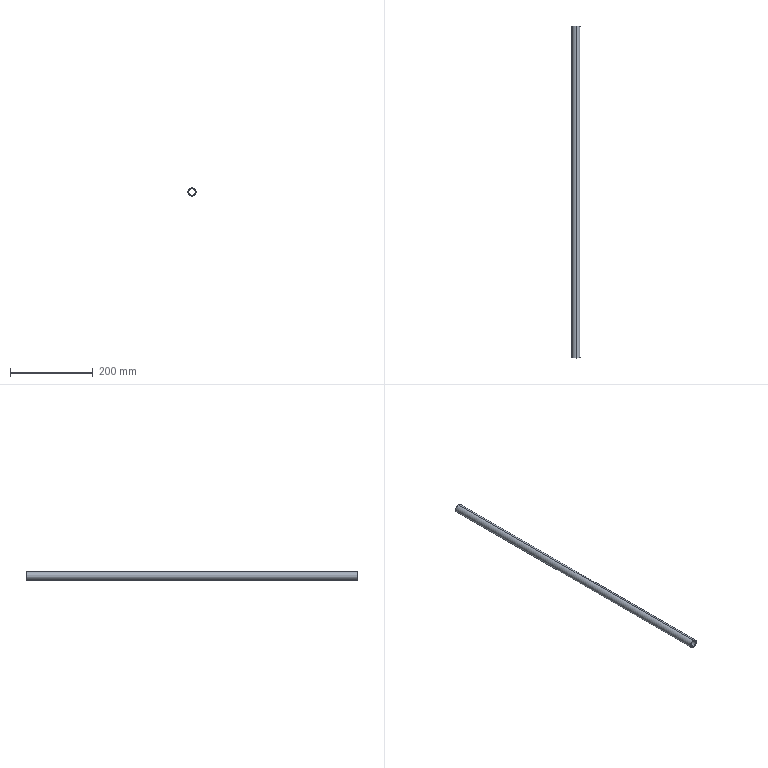Part | SolidWorks | features Sweep 1 | 1 solid | 6 faces | box 20 x 800 x 20 mm | volume 90478 mm3 | cylinder 4 | plane 2 | commonest cylinder face diameters 16 x2 20 x2
STEP:
#1=CARTESIAN_POINT('',(0.,0.,-8.));
#2=VERTEX_POINT('',#1);
#3=CARTESIAN_POINT('',(0.,0.,8.));
#4=VERTEX_POINT('',#3);
#5=CARTESIAN_POINT('',(0.,0.,0.));
#6=DIRECTION('',(0.,1.,0.));
#7=DIRECTION('',(0.,0.,1.));
#8=AXIS2_PLACEMENT_3D('',#5,#6,#7);
#9=CIRCLE('',#8,8.);
#10=EDGE_CURVE('',#2,#4,#9,.T.);
#11=ORIENTED_EDGE('',*,*,#10,.F.);
#12=CARTESIAN_POINT('',(0.,800.,-8.));
#13=VERTEX_POINT('',#12);
#14=CARTESIAN_POINT('',(0.,0.,-8.));
#15=DIRECTION('',(0.,1.,0.));
#16=VECTOR('',#15,1000.);
#17=LINE('',#14,#16);
#18=EDGE_CURVE('',#2,#13,#17,.T.);
#19=ORIENTED_EDGE('',*,*,#18,.T.);
#20=CARTESIAN_POINT('',(0.,800.,8.));
#21=VERTEX_POINT('',#20);
#22=CARTESIAN_POINT('',(0.,800.,0.));
#23=DIRECTION('',(0.,1.,0.));
#24=DIRECTION('',(0.,0.,1.));
#25=AXIS2_PLACEMENT_3D('',#22,#23,#24);
#26=CIRCLE('',#25,8.);
#27=EDGE_CURVE('',#13,#21,#26,.T.);
#28=ORIENTED_EDGE('',*,*,#27,.T.);
#29=CARTESIAN_POINT('',(0.,0.,8.));
#30=DIRECTION('',(0.,1.,0.));
#31=VECTOR('',#30,1000.);
#32=LINE('',#29,#31);
#33=EDGE_CURVE('',#4,#21,#32,.T.);
#34=ORIENTED_EDGE('',*,*,#33,.F.);
#35=EDGE_LOOP('',(#11,#19,#28,#34));
#36=FACE_OUTER_BOUND('',#35,.T.);
#37=CARTESIAN_POINT('',(0.,0.,0.));
#38=DIRECTION('',(0.,1.,0.));
#39=DIRECTION('',(0.,0.,1.));
#40=AXIS2_PLACEMENT_3D('',#37,#38,#39);
#41=CYLINDRICAL_SURFACE('',#40,8.);
#42=ADVANCED_FACE('',(#36),#41,.F.);
#43=CARTESIAN_POINT('',(0.,0.,10.));
#44=VERTEX_POINT('',#43);
#45=CARTESIAN_POINT('',(0.,0.,-10.));
#46=VERTEX_POINT('',#45);
#47=CARTESIAN_POINT('',(0.,0.,0.));
#48=DIRECTION('',(0.,1.,0.));
#49=DIRECTION('',(0.,0.,1.));
#50=AXIS2_PLACEMENT_3D('',#47,#48,#49);
#51=CIRCLE('',#50,10.);
#52=EDGE_CURVE('',#44,#46,#51,.T.);
#53=ORIENTED_EDGE('',*,*,#52,.T.);
#54=CARTESIAN_POINT('',(0.,800.,-10.));
#55=VERTEX_POINT('',#54);
#56=CARTESIAN_POINT('',(0.,0.,-10.));
#57=DIRECTION('',(0.,1.,0.));
#58=VECTOR('',#57,1000.);
#59=LINE('',#56,#58);
#60=EDGE_CURVE('',#46,#55,#59,.T.);
#61=ORIENTED_EDGE('',*,*,#60,.T.);
#62=CARTESIAN_POINT('',(0.,800.,10.));
#63=VERTEX_POINT('',#62);
#64=CARTESIAN_POINT('',(0.,800.,0.));
#65=DIRECTION('',(0.,1.,0.));
#66=DIRECTION('',(0.,0.,1.));
#67=AXIS2_PLACEMENT_3D('',#64,#65,#66);
#68=CIRCLE('',#67,10.);
#69=EDGE_CURVE('',#63,#55,#68,.T.);
#70=ORIENTED_EDGE('',*,*,#69,.F.);
#71=CARTESIAN_POINT('',(0.,0.,10.));
#72=DIRECTION('',(0.,1.,0.));
#73=VECTOR('',#72,1000.);
#74=LINE('',#71,#73);
#75=EDGE_CURVE('',#44,#63,#74,.T.);
#76=ORIENTED_EDGE('',*,*,#75,.F.);
#77=EDGE_LOOP('',(#53,#61,#70,#76));
#78=FACE_OUTER_BOUND('',#77,.T.);
#79=CARTESIAN_POINT('',(0.,0.,0.));
#80=DIRECTION('',(0.,1.,0.));
#81=DIRECTION('',(0.,0.,1.));
#82=AXIS2_PLACEMENT_3D('',#79,#80,#81);
#83=CYLINDRICAL_SURFACE('',#82,10.);
#84=ADVANCED_FACE('',(#78),#83,.T.);
#85=ORIENTED_EDGE('',*,*,#60,.F.);
#86=CARTESIAN_POINT('',(0.,0.,0.));
#87=DIRECTION('',(0.,1.,0.));
#88=DIRECTION('',(0.,0.,1.));
#89=AXIS2_PLACEMENT_3D('',#86,#87,#88);
#90=CIRCLE('',#89,10.);
#91=EDGE_CURVE('',#46,#44,#90,.T.);
#92=ORIENTED_EDGE('',*,*,#91,.T.);
#93=ORIENTED_EDGE('',*,*,#75,.T.);
#94=CARTESIAN_POINT('',(0.,800.,0.));
#95=DIRECTION('',(0.,1.,0.));
#96=DIRECTION('',(0.,0.,1.));
#97=AXIS2_PLACEMENT_3D('',#94,#95,#96);
#98=CIRCLE('',#97,10.);
#99=EDGE_CURVE('',#55,#63,#98,.T.);
#100=ORIENTED_EDGE('',*,*,#99,.F.);
#101=EDGE_LOOP('',(#85,#92,#93,#100));
#102=FACE_OUTER_BOUND('',#101,.T.);
#103=CARTESIAN_POINT('',(0.,0.,0.));
#104=DIRECTION('',(0.,1.,0.));
#105=DIRECTION('',(0.,0.,1.));
#106=AXIS2_PLACEMENT_3D('',#103,#104,#105);
#107=CYLINDRICAL_SURFACE('',#106,10.);
#108=ADVANCED_FACE('',(#102),#107,.T.);
#109=CARTESIAN_POINT('',(0.,800.,0.));
#110=DIRECTION('',(0.,1.,0.));
#111=DIRECTION('',(0.,0.,1.));
#112=AXIS2_PLACEMENT_3D('',#109,#110,#111);
#113=CIRCLE('',#112,8.);
#114=EDGE_CURVE('',#21,#13,#113,.T.);
#115=ORIENTED_EDGE('',*,*,#114,.F.);
#116=ORIENTED_EDGE('',*,*,#27,.F.);
#117=EDGE_LOOP('',(#115,#116));
#118=FACE_BOUND('',#117,.T.);
#119=ORIENTED_EDGE('',*,*,#69,.T.);
#120=ORIENTED_EDGE('',*,*,#99,.T.);
#121=EDGE_LOOP('',(#119,#120));
#122=FACE_OUTER_BOUND('',#121,.T.);
#123=CARTESIAN_POINT('',(0.,800.,0.));
#124=DIRECTION('',(0.,1.,0.));
#125=DIRECTION('',(0.,0.,1.));
#126=AXIS2_PLACEMENT_3D('',#123,#124,#125);
#127=PLANE('',#126);
#128=ADVANCED_FACE('',(#118,#122),#127,.T.);
#129=CARTESIAN_POINT('',(0.,0.,0.));
#130=DIRECTION('',(0.,1.,0.));
#131=DIRECTION('',(0.,0.,1.));
#132=AXIS2_PLACEMENT_3D('',#129,#130,#131);
#133=CIRCLE('',#132,8.);
#134=EDGE_CURVE('',#4,#2,#133,.T.);
#135=ORIENTED_EDGE('',*,*,#134,.T.);
#136=ORIENTED_EDGE('',*,*,#10,.T.);
#137=EDGE_LOOP('',(#135,#136));
#138=FACE_BOUND('',#137,.T.);
#139=ORIENTED_EDGE('',*,*,#52,.F.);
#140=ORIENTED_EDGE('',*,*,#91,.F.);
#141=EDGE_LOOP('',(#139,#140));
#142=FACE_OUTER_BOUND('',#141,.T.);
#143=CARTESIAN_POINT('',(0.,0.,0.));
#144=DIRECTION('',(0.,1.,0.));
#145=DIRECTION('',(0.,0.,1.));
#146=AXIS2_PLACEMENT_3D('',#143,#144,#145);
#147=PLANE('',#146);
#148=ADVANCED_FACE('',(#138,#142),#147,.F.);
#149=ORIENTED_EDGE('',*,*,#18,.F.);
#150=ORIENTED_EDGE('',*,*,#134,.F.);
#151=ORIENTED_EDGE('',*,*,#33,.T.);
#152=ORIENTED_EDGE('',*,*,#114,.T.);
#153=EDGE_LOOP('',(#149,#150,#151,#152));
#154=FACE_OUTER_BOUND('',#153,.T.);
#155=CARTESIAN_POINT('',(0.,0.,0.));
#156=DIRECTION('',(0.,1.,0.));
#157=DIRECTION('',(0.,0.,1.));
#158=AXIS2_PLACEMENT_3D('',#155,#156,#157);
#159=CYLINDRICAL_SURFACE('',#158,8.);
#160=ADVANCED_FACE('',(#154),#159,.F.);
#161=CLOSED_SHELL('',(#42,#84,#108,#128,#148,#160));
#162=MANIFOLD_SOLID_BREP('',#161);
#163=CARTESIAN_POINT('',(0.,0.,0.));
#164=DIRECTION('',(0.,0.,1.));
#165=DIRECTION('',(1.,0.,0.));
#166=AXIS2_PLACEMENT_3D('',#163,#164,#165);
#167=(LENGTH_UNIT()NAMED_UNIT(*)SI_UNIT(.MILLI.,.METRE.));
#168=UNCERTAINTY_MEASURE_WITH_UNIT(LENGTH_MEASURE(0.00001),#167,'','');
#169=(NAMED_UNIT(*)PLANE_ANGLE_UNIT()SI_UNIT($,.RADIAN.));
#170=(NAMED_UNIT(*)SI_UNIT($,.STERADIAN.)SOLID_ANGLE_UNIT());
#171=(GEOMETRIC_REPRESENTATION_CONTEXT(3)GLOBAL_UNCERTAINTY_ASSIGNED_CONTEXT((#168))GLOBAL_UNIT_ASSIGNED_CONTEXT((#167,#169,#170))REPRESENTATION_CONTEXT('',''));
#172=ADVANCED_BREP_SHAPE_REPRESENTATION('',(#162,#166),#171);